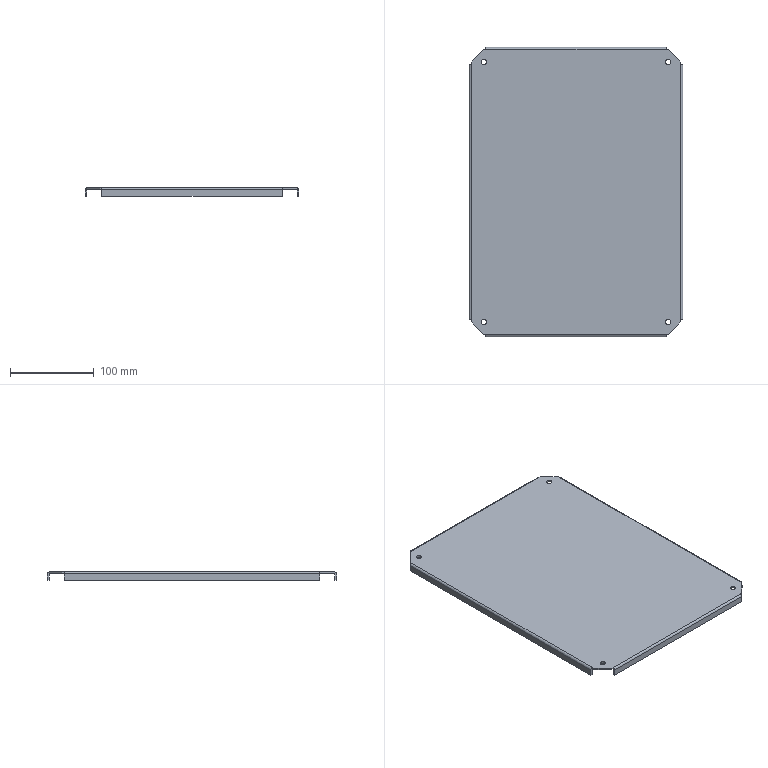Part | SolidWorks | features Chamfer 1, EdgeFlange 1, FlatPattern 1, ICE 1, SMBaseFlange 1, SheetMetal 1 | 1 solid | 58 faces | box 255 x 345 x 10 mm | volume 189359 mm3 | plane 42 | cylinder 16 | commonest cylinder face diameters 6.2 x8 1 x4 5 x4